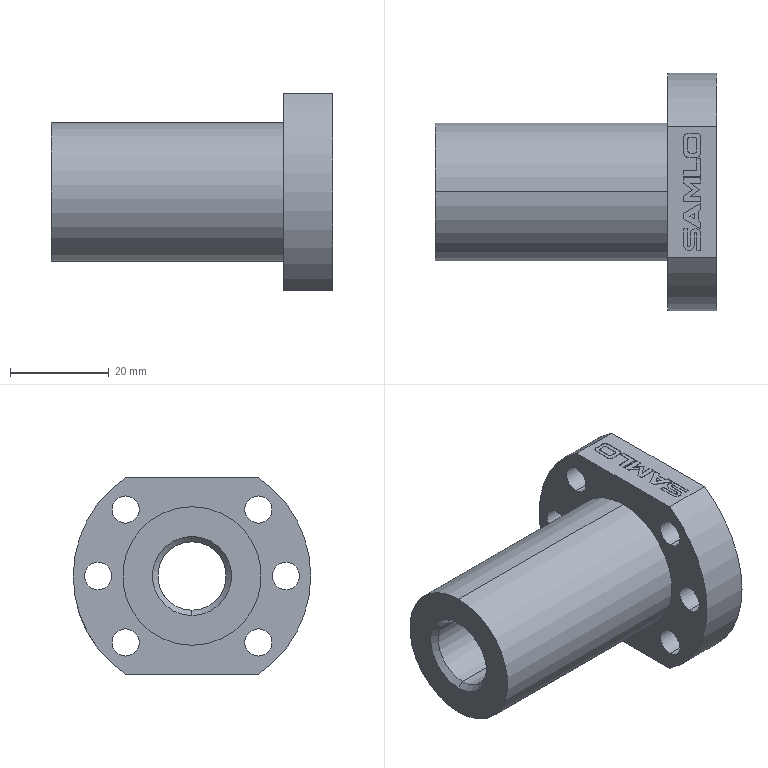Part | SolidWorks | features BaseBody 1 | 1 solid | 95 faces | box 57 x 48 x 40 mm | volume 35215 mm3 | plane 57 | cylinder 32 | cone 6 | commonest cylinder face diameters 5.5 x12 0.804 x4 1.704 x4 0.576 x2 2.113 x2 4.917 x2